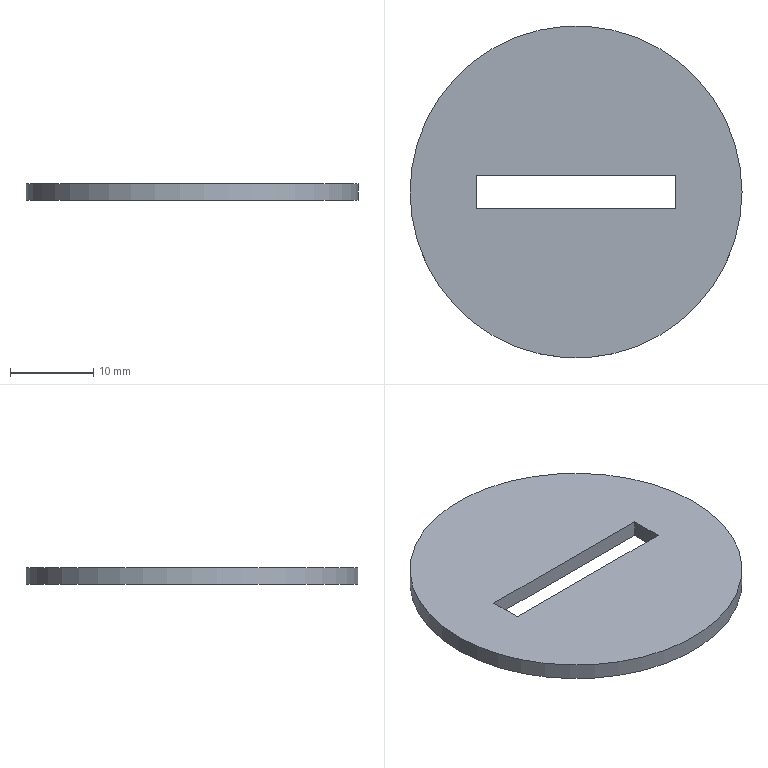Part | NX | features DATUM_CSYS 2, EXTRUDE 1, SKETCH 1 | 1 solid | 7 faces | box 40 x 40 x 2 mm | volume 2321 mm3 | plane 6 | cylinder 1 | commonest cylinder face diameters 40 x1
STEP:
#1=CARTESIAN_POINT('',(-12.,-2.,0.));
#2=VERTEX_POINT('',#1);
#3=CARTESIAN_POINT('',(-12.,2.,0.));
#4=VERTEX_POINT('',#3);
#5=CARTESIAN_POINT('',(-12.,-2.,0.));
#6=DIRECTION('',(0.,1.,0.));
#7=VECTOR('',#6,1000.);
#8=LINE('',#5,#7);
#9=EDGE_CURVE('',#2,#4,#8,.T.);
#10=ORIENTED_EDGE('',*,*,#9,.T.);
#11=CARTESIAN_POINT('',(-12.,2.,2.));
#12=VERTEX_POINT('',#11);
#13=CARTESIAN_POINT('',(-12.,2.,2.));
#14=DIRECTION('',(0.,0.,-1.));
#15=VECTOR('',#14,1000.);
#16=LINE('',#13,#15);
#17=EDGE_CURVE('',#12,#4,#16,.T.);
#18=ORIENTED_EDGE('',*,*,#17,.F.);
#19=CARTESIAN_POINT('',(-12.,-2.,2.));
#20=VERTEX_POINT('',#19);
#21=CARTESIAN_POINT('',(-12.,-2.,2.));
#22=DIRECTION('',(0.,1.,0.));
#23=VECTOR('',#22,1000.);
#24=LINE('',#21,#23);
#25=EDGE_CURVE('',#20,#12,#24,.T.);
#26=ORIENTED_EDGE('',*,*,#25,.F.);
#27=CARTESIAN_POINT('',(-12.,-2.,2.));
#28=DIRECTION('',(0.,0.,-1.));
#29=VECTOR('',#28,1000.);
#30=LINE('',#27,#29);
#31=EDGE_CURVE('',#20,#2,#30,.T.);
#32=ORIENTED_EDGE('',*,*,#31,.T.);
#33=EDGE_LOOP('',(#10,#18,#26,#32));
#34=FACE_BOUND('',#33,.T.);
#35=CARTESIAN_POINT('',(-12.,-2.,2.));
#36=DIRECTION('',(-1.,0.,0.));
#37=DIRECTION('',(0.,-1.,0.));
#38=AXIS2_PLACEMENT_3D('',#35,#36,#37);
#39=PLANE('',#38);
#40=ADVANCED_FACE('',(#34),#39,.F.);
#41=CARTESIAN_POINT('',(12.,2.,0.));
#42=VERTEX_POINT('',#41);
#43=CARTESIAN_POINT('',(-12.,2.,0.));
#44=DIRECTION('',(1.,0.,0.));
#45=VECTOR('',#44,1000.);
#46=LINE('',#43,#45);
#47=EDGE_CURVE('',#4,#42,#46,.T.);
#48=ORIENTED_EDGE('',*,*,#47,.T.);
#49=CARTESIAN_POINT('',(12.,2.,2.));
#50=VERTEX_POINT('',#49);
#51=CARTESIAN_POINT('',(12.,2.,2.));
#52=DIRECTION('',(0.,0.,-1.));
#53=VECTOR('',#52,1000.);
#54=LINE('',#51,#53);
#55=EDGE_CURVE('',#50,#42,#54,.T.);
#56=ORIENTED_EDGE('',*,*,#55,.F.);
#57=CARTESIAN_POINT('',(-12.,2.,2.));
#58=DIRECTION('',(1.,0.,0.));
#59=VECTOR('',#58,1000.);
#60=LINE('',#57,#59);
#61=EDGE_CURVE('',#12,#50,#60,.T.);
#62=ORIENTED_EDGE('',*,*,#61,.F.);
#63=ORIENTED_EDGE('',*,*,#17,.T.);
#64=EDGE_LOOP('',(#48,#56,#62,#63));
#65=FACE_BOUND('',#64,.T.);
#66=CARTESIAN_POINT('',(-12.,2.,2.));
#67=DIRECTION('',(0.,1.,0.));
#68=DIRECTION('',(0.,0.,1.));
#69=AXIS2_PLACEMENT_3D('',#66,#67,#68);
#70=PLANE('',#69);
#71=ADVANCED_FACE('',(#65),#70,.F.);
#72=CARTESIAN_POINT('',(12.,-2.,0.));
#73=VERTEX_POINT('',#72);
#74=CARTESIAN_POINT('',(12.,2.,0.));
#75=DIRECTION('',(0.,-1.,0.));
#76=VECTOR('',#75,1000.);
#77=LINE('',#74,#76);
#78=EDGE_CURVE('',#42,#73,#77,.T.);
#79=ORIENTED_EDGE('',*,*,#78,.T.);
#80=CARTESIAN_POINT('',(12.,-2.,2.));
#81=VERTEX_POINT('',#80);
#82=CARTESIAN_POINT('',(12.,-2.,2.));
#83=DIRECTION('',(0.,0.,-1.));
#84=VECTOR('',#83,1000.);
#85=LINE('',#82,#84);
#86=EDGE_CURVE('',#81,#73,#85,.T.);
#87=ORIENTED_EDGE('',*,*,#86,.F.);
#88=CARTESIAN_POINT('',(12.,2.,2.));
#89=DIRECTION('',(0.,-1.,0.));
#90=VECTOR('',#89,1000.);
#91=LINE('',#88,#90);
#92=EDGE_CURVE('',#50,#81,#91,.T.);
#93=ORIENTED_EDGE('',*,*,#92,.F.);
#94=ORIENTED_EDGE('',*,*,#55,.T.);
#95=EDGE_LOOP('',(#79,#87,#93,#94));
#96=FACE_BOUND('',#95,.T.);
#97=CARTESIAN_POINT('',(12.,2.,2.));
#98=DIRECTION('',(1.,0.,0.));
#99=DIRECTION('',(0.,1.,0.));
#100=AXIS2_PLACEMENT_3D('',#97,#98,#99);
#101=PLANE('',#100);
#102=ADVANCED_FACE('',(#96),#101,.F.);
#103=CARTESIAN_POINT('',(20.,0.,2.));
#104=VERTEX_POINT('',#103);
#105=CARTESIAN_POINT('',(0.,0.,2.));
#106=DIRECTION('',(0.,0.,1.));
#107=DIRECTION('',(1.,0.,0.));
#108=AXIS2_PLACEMENT_3D('',#105,#106,#107);
#109=CIRCLE('',#108,20.);
#110=EDGE_CURVE('',#104,#104,#109,.T.);
#111=ORIENTED_EDGE('',*,*,#110,.F.);
#112=EDGE_LOOP('',(#111));
#113=FACE_BOUND('',#112,.T.);
#114=CARTESIAN_POINT('',(20.,0.,0.));
#115=VERTEX_POINT('',#114);
#116=CARTESIAN_POINT('',(0.,0.,0.));
#117=DIRECTION('',(0.,0.,1.));
#118=DIRECTION('',(1.,0.,0.));
#119=AXIS2_PLACEMENT_3D('',#116,#117,#118);
#120=CIRCLE('',#119,20.);
#121=EDGE_CURVE('',#115,#115,#120,.T.);
#122=ORIENTED_EDGE('',*,*,#121,.T.);
#123=EDGE_LOOP('',(#122));
#124=FACE_BOUND('',#123,.T.);
#125=CARTESIAN_POINT('',(0.,0.,2.));
#126=DIRECTION('',(0.,0.,-1.));
#127=DIRECTION('',(-1.,0.,0.));
#128=AXIS2_PLACEMENT_3D('',#125,#126,#127);
#129=CYLINDRICAL_SURFACE('',#128,20.);
#130=ADVANCED_FACE('',(#113,#124),#129,.T.);
#131=CARTESIAN_POINT('',(12.,-2.,0.));
#132=DIRECTION('',(-1.,0.,0.));
#133=VECTOR('',#132,1000.);
#134=LINE('',#131,#133);
#135=EDGE_CURVE('',#73,#2,#134,.T.);
#136=ORIENTED_EDGE('',*,*,#135,.T.);
#137=ORIENTED_EDGE('',*,*,#31,.F.);
#138=CARTESIAN_POINT('',(12.,-2.,2.));
#139=DIRECTION('',(-1.,0.,0.));
#140=VECTOR('',#139,1000.);
#141=LINE('',#138,#140);
#142=EDGE_CURVE('',#81,#20,#141,.T.);
#143=ORIENTED_EDGE('',*,*,#142,.F.);
#144=ORIENTED_EDGE('',*,*,#86,.T.);
#145=EDGE_LOOP('',(#136,#137,#143,#144));
#146=FACE_BOUND('',#145,.T.);
#147=CARTESIAN_POINT('',(12.,-2.,2.));
#148=DIRECTION('',(0.,-1.,0.));
#149=DIRECTION('',(0.,0.,-1.));
#150=AXIS2_PLACEMENT_3D('',#147,#148,#149);
#151=PLANE('',#150);
#152=ADVANCED_FACE('',(#146),#151,.F.);
#153=ORIENTED_EDGE('',*,*,#110,.T.);
#154=EDGE_LOOP('',(#153));
#155=FACE_BOUND('',#154,.T.);
#156=ORIENTED_EDGE('',*,*,#25,.T.);
#157=ORIENTED_EDGE('',*,*,#61,.T.);
#158=ORIENTED_EDGE('',*,*,#92,.T.);
#159=ORIENTED_EDGE('',*,*,#142,.T.);
#160=EDGE_LOOP('',(#156,#157,#158,#159));
#161=FACE_BOUND('',#160,.T.);
#162=CARTESIAN_POINT('',(0.,0.,2.));
#163=DIRECTION('',(0.,0.,1.));
#164=DIRECTION('',(1.,0.,0.));
#165=AXIS2_PLACEMENT_3D('',#162,#163,#164);
#166=PLANE('',#165);
#167=ADVANCED_FACE('',(#155,#161),#166,.T.);
#168=ORIENTED_EDGE('',*,*,#121,.F.);
#169=EDGE_LOOP('',(#168));
#170=FACE_BOUND('',#169,.T.);
#171=ORIENTED_EDGE('',*,*,#9,.F.);
#172=ORIENTED_EDGE('',*,*,#135,.F.);
#173=ORIENTED_EDGE('',*,*,#78,.F.);
#174=ORIENTED_EDGE('',*,*,#47,.F.);
#175=EDGE_LOOP('',(#171,#172,#173,#174));
#176=FACE_BOUND('',#175,.T.);
#177=CARTESIAN_POINT('',(0.,0.,0.));
#178=DIRECTION('',(0.,0.,1.));
#179=DIRECTION('',(1.,0.,0.));
#180=AXIS2_PLACEMENT_3D('',#177,#178,#179);
#181=PLANE('',#180);
#182=ADVANCED_FACE('',(#170,#176),#181,.F.);
#183=CLOSED_SHELL('',(#40,#71,#102,#130,#152,#167,#182));
#184=MANIFOLD_SOLID_BREP('',#183);
#185=(LENGTH_UNIT()NAMED_UNIT(*)SI_UNIT(.MILLI.,.METRE.));
#186=UNCERTAINTY_MEASURE_WITH_UNIT(LENGTH_MEASURE(0.00001),#185,'','');
#187=(NAMED_UNIT(*)PLANE_ANGLE_UNIT()SI_UNIT($,.RADIAN.));
#188=(NAMED_UNIT(*)SI_UNIT($,.STERADIAN.)SOLID_ANGLE_UNIT());
#189=(GEOMETRIC_REPRESENTATION_CONTEXT(3)GLOBAL_UNCERTAINTY_ASSIGNED_CONTEXT((#186))GLOBAL_UNIT_ASSIGNED_CONTEXT((#185,#187,#188))REPRESENTATION_CONTEXT('',''));
#190=ADVANCED_BREP_SHAPE_REPRESENTATION('',(#184),#189);